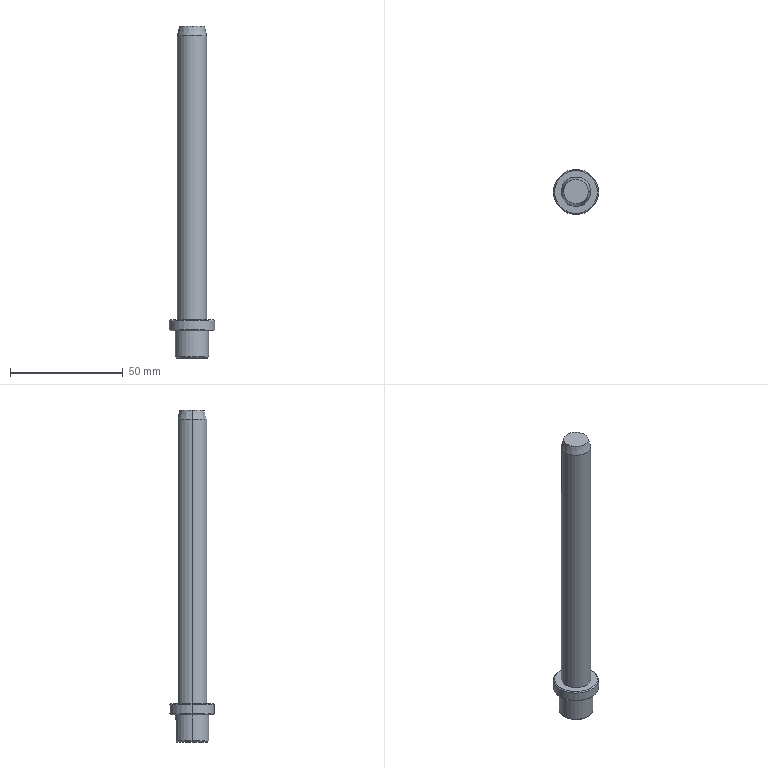Part | STEP file | 11-FG-B05711 | 1 solid | 23 faces | box 20 x 20 x 147 mm | volume 20612 mm3 | cone 9 | cylinder 7 | plane 7 | commonest cylinder face diameters 13 x3 15 x2 20 x2
STEP:
#1=CARTESIAN_POINT('',(9.5,0.,0.));
#2=VERTEX_POINT('',#1);
#3=CARTESIAN_POINT('',(-9.5,0.,0.));
#4=VERTEX_POINT('',#3);
#5=CARTESIAN_POINT('',(0.,0.,0.));
#6=DIRECTION('',(0.,0.,1.));
#7=DIRECTION('',(-1.,0.,0.));
#8=AXIS2_PLACEMENT_3D('',#5,#6,#7);
#9=CIRCLE('',#8,9.5);
#10=EDGE_CURVE('',#2,#4,#9,.T.);
#11=ORIENTED_EDGE('',*,*,#10,.F.);
#12=CARTESIAN_POINT('',(10.,0.,-0.5));
#13=VERTEX_POINT('',#12);
#14=CARTESIAN_POINT('',(10.,0.,-0.5));
#15=DIRECTION('',(0.7071,0.,-0.7071));
#16=VECTOR('',#15,1000.);
#17=LINE('',#14,#16);
#18=EDGE_CURVE('',#2,#13,#17,.T.);
#19=ORIENTED_EDGE('',*,*,#18,.T.);
#20=CARTESIAN_POINT('',(-10.,0.,-0.5));
#21=VERTEX_POINT('',#20);
#22=CARTESIAN_POINT('',(0.,0.,-0.5));
#23=DIRECTION('',(0.,0.,-1.));
#24=DIRECTION('',(-1.,0.,0.));
#25=AXIS2_PLACEMENT_3D('',#22,#23,#24);
#26=CIRCLE('',#25,10.);
#27=EDGE_CURVE('',#21,#13,#26,.T.);
#28=ORIENTED_EDGE('',*,*,#27,.F.);
#29=CARTESIAN_POINT('',(-10.,0.,-0.5));
#30=DIRECTION('',(-0.7071,0.,-0.7071));
#31=VECTOR('',#30,1000.);
#32=LINE('',#29,#31);
#33=EDGE_CURVE('',#4,#21,#32,.T.);
#34=ORIENTED_EDGE('',*,*,#33,.F.);
#35=EDGE_LOOP('',(#11,#19,#28,#34));
#36=FACE_OUTER_BOUND('',#35,.T.);
#37=CARTESIAN_POINT('',(0.,0.,-0.5));
#38=DIRECTION('',(0.,0.,-1.));
#39=DIRECTION('',(-1.,0.,0.));
#40=AXIS2_PLACEMENT_3D('',#37,#38,#39);
#41=CONICAL_SURFACE('',#40,10.,0.7854);
#42=ADVANCED_FACE('',(#36),#41,.T.);
#43=CARTESIAN_POINT('',(-9.5,0.,-5.));
#44=VERTEX_POINT('',#43);
#45=CARTESIAN_POINT('',(9.5,0.,-5.));
#46=VERTEX_POINT('',#45);
#47=CARTESIAN_POINT('',(0.,0.,-5.));
#48=DIRECTION('',(0.,0.,-1.));
#49=DIRECTION('',(-1.,0.,0.));
#50=AXIS2_PLACEMENT_3D('',#47,#48,#49);
#51=CIRCLE('',#50,9.5);
#52=EDGE_CURVE('',#44,#46,#51,.T.);
#53=ORIENTED_EDGE('',*,*,#52,.F.);
#54=CARTESIAN_POINT('',(-10.,0.,-4.5));
#55=VERTEX_POINT('',#54);
#56=CARTESIAN_POINT('',(-9.5,0.,-5.));
#57=DIRECTION('',(-0.7071,0.,0.7071));
#58=VECTOR('',#57,1000.);
#59=LINE('',#56,#58);
#60=EDGE_CURVE('',#44,#55,#59,.T.);
#61=ORIENTED_EDGE('',*,*,#60,.T.);
#62=CARTESIAN_POINT('',(10.,0.,-4.5));
#63=VERTEX_POINT('',#62);
#64=CARTESIAN_POINT('',(0.,0.,-4.5));
#65=DIRECTION('',(0.,0.,1.));
#66=DIRECTION('',(-1.,0.,0.));
#67=AXIS2_PLACEMENT_3D('',#64,#65,#66);
#68=CIRCLE('',#67,10.);
#69=EDGE_CURVE('',#63,#55,#68,.T.);
#70=ORIENTED_EDGE('',*,*,#69,.F.);
#71=CARTESIAN_POINT('',(9.5,0.,-5.));
#72=DIRECTION('',(0.7071,0.,0.7071));
#73=VECTOR('',#72,1000.);
#74=LINE('',#71,#73);
#75=EDGE_CURVE('',#46,#63,#74,.T.);
#76=ORIENTED_EDGE('',*,*,#75,.F.);
#77=EDGE_LOOP('',(#53,#61,#70,#76));
#78=FACE_OUTER_BOUND('',#77,.T.);
#79=CARTESIAN_POINT('',(0.,0.,-5.));
#80=DIRECTION('',(0.,0.,1.));
#81=DIRECTION('',(1.,0.,0.));
#82=AXIS2_PLACEMENT_3D('',#79,#80,#81);
#83=CONICAL_SURFACE('',#82,9.5,0.7854);
#84=ADVANCED_FACE('',(#78),#83,.T.);
#85=CARTESIAN_POINT('',(-7.,0.,-17.));
#86=VERTEX_POINT('',#85);
#87=CARTESIAN_POINT('',(0.,7.,-17.));
#88=VERTEX_POINT('',#87);
#89=CARTESIAN_POINT('',(0.,0.,-17.));
#90=DIRECTION('',(0.,0.,-1.));
#91=DIRECTION('',(-1.,0.,0.));
#92=AXIS2_PLACEMENT_3D('',#89,#90,#91);
#93=CIRCLE('',#92,7.);
#94=EDGE_CURVE('',#86,#88,#93,.T.);
#95=ORIENTED_EDGE('',*,*,#94,.F.);
#96=CARTESIAN_POINT('',(-7.5,0.,-16.5));
#97=VERTEX_POINT('',#96);
#98=CARTESIAN_POINT('',(-7.,0.,-17.));
#99=DIRECTION('',(-0.7071,0.,0.7071));
#100=VECTOR('',#99,1000.);
#101=LINE('',#98,#100);
#102=EDGE_CURVE('',#86,#97,#101,.T.);
#103=ORIENTED_EDGE('',*,*,#102,.T.);
#104=CARTESIAN_POINT('',(-2.693,7.,-16.5));
#105=VERTEX_POINT('',#104);
#106=CARTESIAN_POINT('',(0.,0.,-16.5));
#107=DIRECTION('',(0.,0.,1.));
#108=DIRECTION('',(-1.,0.,0.));
#109=AXIS2_PLACEMENT_3D('',#106,#107,#108);
#110=CIRCLE('',#109,7.5);
#111=EDGE_CURVE('',#105,#97,#110,.T.);
#112=ORIENTED_EDGE('',*,*,#111,.F.);
#113=CARTESIAN_POINT('',(0.,7.,-17.));
#114=CARTESIAN_POINT('',(-0.4603,7.,-17.));
#115=CARTESIAN_POINT('',(-0.9154,7.,-16.954));
#116=CARTESIAN_POINT('',(-1.816,7.,-16.782));
#117=CARTESIAN_POINT('',(-2.263,7.,-16.654));
#118=CARTESIAN_POINT('',(-2.693,7.,-16.5));
#119=B_SPLINE_CURVE_WITH_KNOTS('',3,(#113,#114,#115,#116,#117,#118),.UNSPECIFIED.,.F.,.F.,(4,2,4),(0.008783,0.01014,0.0115),.UNSPECIFIED.);
#120=EDGE_CURVE('',#88,#105,#119,.T.);
#121=ORIENTED_EDGE('',*,*,#120,.F.);
#122=EDGE_LOOP('',(#95,#103,#112,#121));
#123=FACE_OUTER_BOUND('',#122,.T.);
#124=CARTESIAN_POINT('',(0.,0.,-17.));
#125=DIRECTION('',(0.,0.,1.));
#126=DIRECTION('',(1.,0.,0.));
#127=AXIS2_PLACEMENT_3D('',#124,#125,#126);
#128=CONICAL_SURFACE('',#127,7.,0.7854);
#129=ADVANCED_FACE('',(#123),#128,.T.);
#130=ORIENTED_EDGE('',*,*,#102,.F.);
#131=CARTESIAN_POINT('',(7.,0.,-17.));
#132=VERTEX_POINT('',#131);
#133=CARTESIAN_POINT('',(0.,0.,-17.));
#134=DIRECTION('',(0.,0.,-1.));
#135=DIRECTION('',(-1.,0.,0.));
#136=AXIS2_PLACEMENT_3D('',#133,#134,#135);
#137=CIRCLE('',#136,7.);
#138=EDGE_CURVE('',#132,#86,#137,.T.);
#139=ORIENTED_EDGE('',*,*,#138,.F.);
#140=CARTESIAN_POINT('',(7.5,0.,-16.5));
#141=VERTEX_POINT('',#140);
#142=CARTESIAN_POINT('',(7.,0.,-17.));
#143=DIRECTION('',(0.7071,0.,0.7071));
#144=VECTOR('',#143,1000.);
#145=LINE('',#142,#144);
#146=EDGE_CURVE('',#132,#141,#145,.T.);
#147=ORIENTED_EDGE('',*,*,#146,.T.);
#148=CARTESIAN_POINT('',(0.,0.,-16.5));
#149=DIRECTION('',(0.,0.,1.));
#150=DIRECTION('',(-1.,0.,0.));
#151=AXIS2_PLACEMENT_3D('',#148,#149,#150);
#152=CIRCLE('',#151,7.5);
#153=EDGE_CURVE('',#97,#141,#152,.T.);
#154=ORIENTED_EDGE('',*,*,#153,.F.);
#155=EDGE_LOOP('',(#130,#139,#147,#154));
#156=FACE_OUTER_BOUND('',#155,.T.);
#157=CARTESIAN_POINT('',(0.,0.,-17.));
#158=DIRECTION('',(0.,0.,1.));
#159=DIRECTION('',(1.,0.,0.));
#160=AXIS2_PLACEMENT_3D('',#157,#158,#159);
#161=CONICAL_SURFACE('',#160,7.,0.7854);
#162=ADVANCED_FACE('',(#156),#161,.T.);
#163=ORIENTED_EDGE('',*,*,#111,.T.);
#164=CARTESIAN_POINT('',(-7.5,0.,-5.));
#165=VERTEX_POINT('',#164);
#166=CARTESIAN_POINT('',(-7.5,0.,-17.));
#167=DIRECTION('',(0.,0.,1.));
#168=VECTOR('',#167,1000.);
#169=LINE('',#166,#168);
#170=EDGE_CURVE('',#97,#165,#169,.T.);
#171=ORIENTED_EDGE('',*,*,#170,.T.);
#172=CARTESIAN_POINT('',(7.5,0.,-5.));
#173=VERTEX_POINT('',#172);
#174=CARTESIAN_POINT('',(0.,0.,-5.));
#175=DIRECTION('',(0.,0.,-1.));
#176=DIRECTION('',(-1.,0.,0.));
#177=AXIS2_PLACEMENT_3D('',#174,#175,#176);
#178=CIRCLE('',#177,7.5);
#179=EDGE_CURVE('',#165,#173,#178,.T.);
#180=ORIENTED_EDGE('',*,*,#179,.T.);
#181=CARTESIAN_POINT('',(7.5,0.,-17.));
#182=DIRECTION('',(0.,0.,1.));
#183=VECTOR('',#182,1000.);
#184=LINE('',#181,#183);
#185=EDGE_CURVE('',#141,#173,#184,.T.);
#186=ORIENTED_EDGE('',*,*,#185,.F.);
#187=CARTESIAN_POINT('',(2.693,7.,-16.5));
#188=VERTEX_POINT('',#187);
#189=CARTESIAN_POINT('',(0.,0.,-16.5));
#190=DIRECTION('',(0.,0.,1.));
#191=DIRECTION('',(-1.,0.,0.));
#192=AXIS2_PLACEMENT_3D('',#189,#190,#191);
#193=CIRCLE('',#192,7.5);
#194=EDGE_CURVE('',#141,#188,#193,.T.);
#195=ORIENTED_EDGE('',*,*,#194,.T.);
#196=CARTESIAN_POINT('',(2.693,7.,-7.));
#197=VERTEX_POINT('',#196);
#198=CARTESIAN_POINT('',(2.693,7.,-17.));
#199=DIRECTION('',(0.,0.,1.));
#200=VECTOR('',#199,1000.);
#201=LINE('',#198,#200);
#202=EDGE_CURVE('',#188,#197,#201,.T.);
#203=ORIENTED_EDGE('',*,*,#202,.T.);
#204=CARTESIAN_POINT('',(-2.693,7.,-7.));
#205=VERTEX_POINT('',#204);
#206=CARTESIAN_POINT('',(0.,0.,-7.));
#207=DIRECTION('',(0.,0.,-1.));
#208=DIRECTION('',(-1.,0.,0.));
#209=AXIS2_PLACEMENT_3D('',#206,#207,#208);
#210=CIRCLE('',#209,7.5);
#211=EDGE_CURVE('',#205,#197,#210,.T.);
#212=ORIENTED_EDGE('',*,*,#211,.F.);
#213=CARTESIAN_POINT('',(-2.693,7.,-17.));
#214=DIRECTION('',(0.,0.,-1.));
#215=VECTOR('',#214,1000.);
#216=LINE('',#213,#215);
#217=EDGE_CURVE('',#205,#105,#216,.T.);
#218=ORIENTED_EDGE('',*,*,#217,.T.);
#219=EDGE_LOOP('',(#163,#171,#180,#186,#195,#203,#212,#218));
#220=FACE_OUTER_BOUND('',#219,.T.);
#221=CARTESIAN_POINT('',(0.,0.,-17.));
#222=DIRECTION('',(0.,0.,1.));
#223=DIRECTION('',(1.,0.,0.));
#224=AXIS2_PLACEMENT_3D('',#221,#222,#223);
#225=CYLINDRICAL_SURFACE('',#224,7.5);
#226=ADVANCED_FACE('',(#220),#225,.T.);
#227=ORIENTED_EDGE('',*,*,#69,.T.);
#228=CARTESIAN_POINT('',(-10.,0.,-5.));
#229=DIRECTION('',(0.,0.,1.));
#230=VECTOR('',#229,1000.);
#231=LINE('',#228,#230);
#232=EDGE_CURVE('',#55,#21,#231,.T.);
#233=ORIENTED_EDGE('',*,*,#232,.T.);
#234=ORIENTED_EDGE('',*,*,#27,.T.);
#235=CARTESIAN_POINT('',(10.,0.,-5.));
#236=DIRECTION('',(0.,0.,1.));
#237=VECTOR('',#236,1000.);
#238=LINE('',#235,#237);
#239=EDGE_CURVE('',#63,#13,#238,.T.);
#240=ORIENTED_EDGE('',*,*,#239,.F.);
#241=EDGE_LOOP('',(#227,#233,#234,#240));
#242=FACE_OUTER_BOUND('',#241,.T.);
#243=CARTESIAN_POINT('',(0.,0.,-5.));
#244=DIRECTION('',(0.,0.,1.));
#245=DIRECTION('',(1.,0.,0.));
#246=AXIS2_PLACEMENT_3D('',#243,#244,#245);
#247=CYLINDRICAL_SURFACE('',#246,10.);
#248=ADVANCED_FACE('',(#242),#247,.T.);
#249=CARTESIAN_POINT('',(5.428,0.,130.));
#250=VERTEX_POINT('',#249);
#251=CARTESIAN_POINT('',(-5.428,0.,130.));
#252=VERTEX_POINT('',#251);
#253=CARTESIAN_POINT('',(0.,0.,130.));
#254=DIRECTION('',(0.,0.,1.));
#255=DIRECTION('',(1.,0.,0.));
#256=AXIS2_PLACEMENT_3D('',#253,#254,#255);
#257=CIRCLE('',#256,5.428);
#258=EDGE_CURVE('',#250,#252,#257,.T.);
#259=ORIENTED_EDGE('',*,*,#258,.F.);
#260=CARTESIAN_POINT('',(6.5,0.,126.));
#261=VERTEX_POINT('',#260);
#262=CARTESIAN_POINT('',(5.428,0.,130.));
#263=DIRECTION('',(0.2588,0.,-0.9659));
#264=VECTOR('',#263,1000.);
#265=LINE('',#262,#264);
#266=EDGE_CURVE('',#250,#261,#265,.T.);
#267=ORIENTED_EDGE('',*,*,#266,.T.);
#268=CARTESIAN_POINT('',(2.5,6.,126.));
#269=VERTEX_POINT('',#268);
#270=CARTESIAN_POINT('',(0.,0.,126.));
#271=DIRECTION('',(0.,0.,-1.));
#272=DIRECTION('',(1.,0.,0.));
#273=AXIS2_PLACEMENT_3D('',#270,#271,#272);
#274=CIRCLE('',#273,6.5);
#275=EDGE_CURVE('',#269,#261,#274,.T.);
#276=ORIENTED_EDGE('',*,*,#275,.F.);
#277=CARTESIAN_POINT('',(-2.5,6.,126.));
#278=VERTEX_POINT('',#277);
#279=CARTESIAN_POINT('',(2.5,6.,126.));
#280=CARTESIAN_POINT('',(2.346,6.,126.221));
#281=CARTESIAN_POINT('',(2.185,6.,126.435));
#282=CARTESIAN_POINT('',(1.84,6.,126.844));
#283=CARTESIAN_POINT('',(1.657,6.,127.039));
#284=CARTESIAN_POINT('',(1.253,6.,127.395));
#285=CARTESIAN_POINT('',(1.031,6.,127.556));
#286=CARTESIAN_POINT('',(0.6671,6.,127.733));
#287=CARTESIAN_POINT('',(0.5384,6.,127.781));
#288=CARTESIAN_POINT('',(0.2764,6.,127.848));
#289=CARTESIAN_POINT('',(0.1417,6.,127.866));
#290=CARTESIAN_POINT('',(-0.1312,6.,127.866));
#291=CARTESIAN_POINT('',(-0.265,6.,127.85));
#292=CARTESIAN_POINT('',(-0.5279,6.,127.785));
#293=CARTESIAN_POINT('',(-0.6568,6.,127.737));
#294=CARTESIAN_POINT('',(-1.022,6.,127.561));
#295=CARTESIAN_POINT('',(-1.245,6.,127.401));
#296=CARTESIAN_POINT('',(-1.65,6.,127.046));
#297=CARTESIAN_POINT('',(-1.835,6.,126.85));
#298=CARTESIAN_POINT('',(-2.184,6.,126.437));
#299=CARTESIAN_POINT('',(-2.346,6.,126.221));
#300=CARTESIAN_POINT('',(-2.5,6.,126.));
#301=B_SPLINE_CURVE_WITH_KNOTS('',3,(#279,#280,#281,#282,#283,#284,#285,#286,#287,#288,#289,#290,#291,#292,#293,#294,#295,#296,#297,#298,#299,#300),.UNSPECIFIED.,.F.,.F.,(4,2,2,2,2,2,2,2,2,2,4),(0.007754,0.008553,0.009351,0.01015,0.01055,0.01095,0.01135,0.01175,0.01254,0.01334,0.01414),.UNSPECIFIED.);
#302=EDGE_CURVE('',#269,#278,#301,.T.);
#303=ORIENTED_EDGE('',*,*,#302,.T.);
#304=CARTESIAN_POINT('',(-6.5,0.,126.));
#305=VERTEX_POINT('',#304);
#306=CARTESIAN_POINT('',(0.,0.,126.));
#307=DIRECTION('',(0.,0.,-1.));
#308=DIRECTION('',(1.,0.,0.));
#309=AXIS2_PLACEMENT_3D('',#306,#307,#308);
#310=CIRCLE('',#309,6.5);
#311=EDGE_CURVE('',#305,#278,#310,.T.);
#312=ORIENTED_EDGE('',*,*,#311,.F.);
#313=CARTESIAN_POINT('',(-5.428,0.,130.));
#314=DIRECTION('',(-0.2588,0.,-0.9659));
#315=VECTOR('',#314,1000.);
#316=LINE('',#313,#315);
#317=EDGE_CURVE('',#252,#305,#316,.T.);
#318=ORIENTED_EDGE('',*,*,#317,.F.);
#319=EDGE_LOOP('',(#259,#267,#276,#303,#312,#318));
#320=FACE_OUTER_BOUND('',#319,.T.);
#321=CARTESIAN_POINT('',(0.,0.,130.));
#322=DIRECTION('',(0.,0.,-1.));
#323=DIRECTION('',(-1.,0.,0.));
#324=AXIS2_PLACEMENT_3D('',#321,#322,#323);
#325=CONICAL_SURFACE('',#324,5.428,0.2618);
#326=ADVANCED_FACE('',(#320),#325,.T.);
#327=ORIENTED_EDGE('',*,*,#275,.T.);
#328=CARTESIAN_POINT('',(6.5,0.,0.));
#329=VERTEX_POINT('',#328);
#330=CARTESIAN_POINT('',(6.5,0.,130.));
#331=DIRECTION('',(0.,0.,-1.));
#332=VECTOR('',#331,1000.);
#333=LINE('',#330,#332);
#334=EDGE_CURVE('',#261,#329,#333,.T.);
#335=ORIENTED_EDGE('',*,*,#334,.T.);
#336=CARTESIAN_POINT('',(2.5,6.,0.));
#337=VERTEX_POINT('',#336);
#338=CARTESIAN_POINT('',(0.,0.,0.));
#339=DIRECTION('',(0.,0.,-1.));
#340=DIRECTION('',(-1.,0.,0.));
#341=AXIS2_PLACEMENT_3D('',#338,#339,#340);
#342=CIRCLE('',#341,6.5);
#343=EDGE_CURVE('',#337,#329,#342,.T.);
#344=ORIENTED_EDGE('',*,*,#343,.F.);
#345=CARTESIAN_POINT('',(2.5,6.,130.));
#346=DIRECTION('',(0.,0.,-1.));
#347=VECTOR('',#346,1000.);
#348=LINE('',#345,#347);
#349=EDGE_CURVE('',#269,#337,#348,.T.);
#350=ORIENTED_EDGE('',*,*,#349,.F.);
#351=EDGE_LOOP('',(#327,#335,#344,#350));
#352=FACE_OUTER_BOUND('',#351,.T.);
#353=CARTESIAN_POINT('',(0.,0.,130.));
#354=DIRECTION('',(0.,0.,-1.));
#355=DIRECTION('',(-1.,0.,0.));
#356=AXIS2_PLACEMENT_3D('',#353,#354,#355);
#357=CYLINDRICAL_SURFACE('',#356,6.5);
#358=ADVANCED_FACE('',(#352),#357,.T.);
#359=ORIENTED_EDGE('',*,*,#334,.F.);
#360=CARTESIAN_POINT('',(0.,0.,126.));
#361=DIRECTION('',(0.,0.,-1.));
#362=DIRECTION('',(1.,0.,0.));
#363=AXIS2_PLACEMENT_3D('',#360,#361,#362);
#364=CIRCLE('',#363,6.5);
#365=EDGE_CURVE('',#261,#305,#364,.T.);
#366=ORIENTED_EDGE('',*,*,#365,.T.);
#367=CARTESIAN_POINT('',(-6.5,0.,0.));
#368=VERTEX_POINT('',#367);
#369=CARTESIAN_POINT('',(-6.5,0.,130.));
#370=DIRECTION('',(0.,0.,-1.));
#371=VECTOR('',#370,1000.);
#372=LINE('',#369,#371);
#373=EDGE_CURVE('',#305,#368,#372,.T.);
#374=ORIENTED_EDGE('',*,*,#373,.T.);
#375=CARTESIAN_POINT('',(0.,0.,0.));
#376=DIRECTION('',(0.,0.,-1.));
#377=DIRECTION('',(-1.,0.,0.));
#378=AXIS2_PLACEMENT_3D('',#375,#376,#377);
#379=CIRCLE('',#378,6.5);
#380=EDGE_CURVE('',#329,#368,#379,.T.);
#381=ORIENTED_EDGE('',*,*,#380,.F.);
#382=EDGE_LOOP('',(#359,#366,#374,#381));
#383=FACE_OUTER_BOUND('',#382,.T.);
#384=CARTESIAN_POINT('',(0.,0.,130.));
#385=DIRECTION('',(0.,0.,-1.));
#386=DIRECTION('',(-1.,0.,0.));
#387=AXIS2_PLACEMENT_3D('',#384,#385,#386);
#388=CYLINDRICAL_SURFACE('',#387,6.5);
#389=ADVANCED_FACE('',(#383),#388,.T.);
#390=ORIENTED_EDGE('',*,*,#373,.F.);
#391=ORIENTED_EDGE('',*,*,#311,.T.);
#392=CARTESIAN_POINT('',(-2.5,6.,0.));
#393=VERTEX_POINT('',#392);
#394=CARTESIAN_POINT('',(-2.5,6.,130.));
#395=DIRECTION('',(0.,0.,1.));
#396=VECTOR('',#395,1000.);
#397=LINE('',#394,#396);
#398=EDGE_CURVE('',#393,#278,#397,.T.);
#399=ORIENTED_EDGE('',*,*,#398,.F.);
#400=CARTESIAN_POINT('',(0.,0.,0.));
#401=DIRECTION('',(0.,0.,-1.));
#402=DIRECTION('',(-1.,0.,0.));
#403=AXIS2_PLACEMENT_3D('',#400,#401,#402);
#404=CIRCLE('',#403,6.5);
#405=EDGE_CURVE('',#368,#393,#404,.T.);
#406=ORIENTED_EDGE('',*,*,#405,.F.);
#407=EDGE_LOOP('',(#390,#391,#399,#406));
#408=FACE_OUTER_BOUND('',#407,.T.);
#409=CARTESIAN_POINT('',(0.,0.,130.));
#410=DIRECTION('',(0.,0.,-1.));
#411=DIRECTION('',(-1.,0.,0.));
#412=AXIS2_PLACEMENT_3D('',#409,#410,#411);
#413=CYLINDRICAL_SURFACE('',#412,6.5);
#414=ADVANCED_FACE('',(#408),#413,.T.);
#415=ORIENTED_EDGE('',*,*,#266,.F.);
#416=CARTESIAN_POINT('',(0.,0.,130.));
#417=DIRECTION('',(0.,0.,1.));
#418=DIRECTION('',(1.,0.,0.));
#419=AXIS2_PLACEMENT_3D('',#416,#417,#418);
#420=CIRCLE('',#419,5.428);
#421=EDGE_CURVE('',#252,#250,#420,.T.);
#422=ORIENTED_EDGE('',*,*,#421,.F.);
#423=ORIENTED_EDGE('',*,*,#317,.T.);
#424=ORIENTED_EDGE('',*,*,#365,.F.);
#425=EDGE_LOOP('',(#415,#422,#423,#424));
#426=FACE_OUTER_BOUND('',#425,.T.);
#427=CARTESIAN_POINT('',(0.,0.,130.));
#428=DIRECTION('',(0.,0.,-1.));
#429=DIRECTION('',(-1.,0.,0.));
#430=AXIS2_PLACEMENT_3D('',#427,#428,#429);
#431=CONICAL_SURFACE('',#430,5.428,0.2618);
#432=ADVANCED_FACE('',(#426),#431,.T.);
#433=CARTESIAN_POINT('',(0.,0.,-5.));
#434=DIRECTION('',(0.,0.,-1.));
#435=DIRECTION('',(-1.,0.,0.));
#436=AXIS2_PLACEMENT_3D('',#433,#434,#435);
#437=CIRCLE('',#436,9.5);
#438=EDGE_CURVE('',#46,#44,#437,.T.);
#439=ORIENTED_EDGE('',*,*,#438,.T.);
#440=ORIENTED_EDGE('',*,*,#52,.T.);
#441=EDGE_LOOP('',(#439,#440));
#442=FACE_OUTER_BOUND('',#441,.T.);
#443=CARTESIAN_POINT('',(0.,0.,-5.));
#444=DIRECTION('',(0.,0.,-1.));
#445=DIRECTION('',(-1.,0.,0.));
#446=AXIS2_PLACEMENT_3D('',#443,#444,#445);
#447=CIRCLE('',#446,7.5);
#448=EDGE_CURVE('',#173,#165,#447,.T.);
#449=ORIENTED_EDGE('',*,*,#448,.F.);
#450=ORIENTED_EDGE('',*,*,#179,.F.);
#451=EDGE_LOOP('',(#449,#450));
#452=FACE_BOUND('',#451,.T.);
#453=CARTESIAN_POINT('',(0.,0.,-5.));
#454=DIRECTION('',(0.,0.,-1.));
#455=DIRECTION('',(-1.,0.,0.));
#456=AXIS2_PLACEMENT_3D('',#453,#454,#455);
#457=PLANE('',#456);
#458=ADVANCED_FACE('',(#442,#452),#457,.T.);
#459=ORIENTED_EDGE('',*,*,#421,.T.);
#460=ORIENTED_EDGE('',*,*,#258,.T.);
#461=EDGE_LOOP('',(#459,#460));
#462=FACE_OUTER_BOUND('',#461,.T.);
#463=CARTESIAN_POINT('',(0.,0.,130.));
#464=DIRECTION('',(0.,0.,1.));
#465=DIRECTION('',(1.,0.,0.));
#466=AXIS2_PLACEMENT_3D('',#463,#464,#465);
#467=PLANE('',#466);
#468=ADVANCED_FACE('',(#462),#467,.T.);
#469=CARTESIAN_POINT('',(0.,0.,0.));
#470=DIRECTION('',(0.,0.,1.));
#471=DIRECTION('',(-1.,0.,0.));
#472=AXIS2_PLACEMENT_3D('',#469,#470,#471);
#473=CIRCLE('',#472,9.5);
#474=EDGE_CURVE('',#4,#2,#473,.T.);
#475=ORIENTED_EDGE('',*,*,#474,.T.);
#476=ORIENTED_EDGE('',*,*,#10,.T.);
#477=EDGE_LOOP('',(#475,#476));
#478=FACE_OUTER_BOUND('',#477,.T.);
#479=ORIENTED_EDGE('',*,*,#343,.T.);
#480=ORIENTED_EDGE('',*,*,#380,.T.);
#481=ORIENTED_EDGE('',*,*,#405,.T.);
#482=CARTESIAN_POINT('',(-7.766,6.,0.));
#483=DIRECTION('',(1.,0.,0.));
#484=VECTOR('',#483,1000.);
#485=LINE('',#482,#484);
#486=EDGE_CURVE('',#393,#337,#485,.T.);
#487=ORIENTED_EDGE('',*,*,#486,.T.);
#488=EDGE_LOOP('',(#479,#480,#481,#487));
#489=FACE_BOUND('',#488,.T.);
#490=CARTESIAN_POINT('',(0.,0.,0.));
#491=DIRECTION('',(0.,0.,-1.));
#492=DIRECTION('',(-1.,0.,0.));
#493=AXIS2_PLACEMENT_3D('',#490,#491,#492);
#494=PLANE('',#493);
#495=ADVANCED_FACE('',(#478,#489),#494,.F.);
#496=ORIENTED_EDGE('',*,*,#232,.F.);
#497=CARTESIAN_POINT('',(0.,0.,-4.5));
#498=DIRECTION('',(0.,0.,1.));
#499=DIRECTION('',(-1.,0.,0.));
#500=AXIS2_PLACEMENT_3D('',#497,#498,#499);
#501=CIRCLE('',#500,10.);
#502=EDGE_CURVE('',#55,#63,#501,.T.);
#503=ORIENTED_EDGE('',*,*,#502,.T.);
#504=ORIENTED_EDGE('',*,*,#239,.T.);
#505=CARTESIAN_POINT('',(0.,0.,-0.5));
#506=DIRECTION('',(0.,0.,-1.));
#507=DIRECTION('',(-1.,0.,0.));
#508=AXIS2_PLACEMENT_3D('',#505,#506,#507);
#509=CIRCLE('',#508,10.);
#510=EDGE_CURVE('',#13,#21,#509,.T.);
#511=ORIENTED_EDGE('',*,*,#510,.T.);
#512=EDGE_LOOP('',(#496,#503,#504,#511));
#513=FACE_OUTER_BOUND('',#512,.T.);
#514=CARTESIAN_POINT('',(0.,0.,-5.));
#515=DIRECTION('',(0.,0.,1.));
#516=DIRECTION('',(1.,0.,0.));
#517=AXIS2_PLACEMENT_3D('',#514,#515,#516);
#518=CYLINDRICAL_SURFACE('',#517,10.);
#519=ADVANCED_FACE('',(#513),#518,.T.);
#520=ORIENTED_EDGE('',*,*,#170,.F.);
#521=ORIENTED_EDGE('',*,*,#153,.T.);
#522=ORIENTED_EDGE('',*,*,#185,.T.);
#523=ORIENTED_EDGE('',*,*,#448,.T.);
#524=EDGE_LOOP('',(#520,#521,#522,#523));
#525=FACE_OUTER_BOUND('',#524,.T.);
#526=CARTESIAN_POINT('',(0.,0.,-17.));
#527=DIRECTION('',(0.,0.,1.));
#528=DIRECTION('',(1.,0.,0.));
#529=AXIS2_PLACEMENT_3D('',#526,#527,#528);
#530=CYLINDRICAL_SURFACE('',#529,7.5);
#531=ADVANCED_FACE('',(#525),#530,.T.);
#532=CARTESIAN_POINT('',(0.,0.,-17.));
#533=DIRECTION('',(0.,0.,-1.));
#534=DIRECTION('',(-1.,0.,0.));
#535=AXIS2_PLACEMENT_3D('',#532,#533,#534);
#536=CIRCLE('',#535,7.);
#537=EDGE_CURVE('',#88,#132,#536,.T.);
#538=ORIENTED_EDGE('',*,*,#537,.T.);
#539=ORIENTED_EDGE('',*,*,#138,.T.);
#540=ORIENTED_EDGE('',*,*,#94,.T.);
#541=EDGE_LOOP('',(#538,#539,#540));
#542=FACE_OUTER_BOUND('',#541,.T.);
#543=CARTESIAN_POINT('',(0.,0.,-17.));
#544=DIRECTION('',(0.,0.,-1.));
#545=DIRECTION('',(-1.,0.,0.));
#546=AXIS2_PLACEMENT_3D('',#543,#544,#545);
#547=PLANE('',#546);
#548=ADVANCED_FACE('',(#542),#547,.T.);
#549=ORIENTED_EDGE('',*,*,#349,.T.);
#550=ORIENTED_EDGE('',*,*,#486,.F.);
#551=ORIENTED_EDGE('',*,*,#398,.T.);
#552=ORIENTED_EDGE('',*,*,#302,.F.);
#553=EDGE_LOOP('',(#549,#550,#551,#552));
#554=FACE_OUTER_BOUND('',#553,.T.);
#555=CARTESIAN_POINT('',(-7.766,6.,130.));
#556=DIRECTION('',(0.,1.,0.));
#557=DIRECTION('',(0.,0.,1.));
#558=AXIS2_PLACEMENT_3D('',#555,#556,#557);
#559=PLANE('',#558);
#560=ADVANCED_FACE('',(#554),#559,.T.);
#561=ORIENTED_EDGE('',*,*,#146,.F.);
#562=ORIENTED_EDGE('',*,*,#537,.F.);
#563=CARTESIAN_POINT('',(2.693,7.,-16.5));
#564=CARTESIAN_POINT('',(2.258,7.,-16.656));
#565=CARTESIAN_POINT('',(1.818,7.,-16.781));
#566=CARTESIAN_POINT('',(1.145,7.,-16.91));
#567=CARTESIAN_POINT('',(0.919,7.,-16.944));
#568=CARTESIAN_POINT('',(0.4621,7.,-16.988));
#569=CARTESIAN_POINT('',(0.2303,7.,-17.));
#570=CARTESIAN_POINT('',(0.,7.,-17.));
#571=B_SPLINE_CURVE_WITH_KNOTS('',3,(#563,#564,#565,#566,#567,#568,#569,#570),.UNSPECIFIED.,.F.,.F.,(4,2,2,4),(0.006062,0.007422,0.008103,0.008783),.UNSPECIFIED.);
#572=EDGE_CURVE('',#188,#88,#571,.T.);
#573=ORIENTED_EDGE('',*,*,#572,.F.);
#574=ORIENTED_EDGE('',*,*,#194,.F.);
#575=EDGE_LOOP('',(#561,#562,#573,#574));
#576=FACE_OUTER_BOUND('',#575,.T.);
#577=CARTESIAN_POINT('',(0.,0.,-17.));
#578=DIRECTION('',(0.,0.,1.));
#579=DIRECTION('',(1.,0.,0.));
#580=AXIS2_PLACEMENT_3D('',#577,#578,#579);
#581=CONICAL_SURFACE('',#580,7.,0.7854);
#582=ADVANCED_FACE('',(#576),#581,.T.);
#583=ORIENTED_EDGE('',*,*,#60,.F.);
#584=ORIENTED_EDGE('',*,*,#438,.F.);
#585=ORIENTED_EDGE('',*,*,#75,.T.);
#586=ORIENTED_EDGE('',*,*,#502,.F.);
#587=EDGE_LOOP('',(#583,#584,#585,#586));
#588=FACE_OUTER_BOUND('',#587,.T.);
#589=CARTESIAN_POINT('',(0.,0.,-5.));
#590=DIRECTION('',(0.,0.,1.));
#591=DIRECTION('',(1.,0.,0.));
#592=AXIS2_PLACEMENT_3D('',#589,#590,#591);
#593=CONICAL_SURFACE('',#592,9.5,0.7854);
#594=ADVANCED_FACE('',(#588),#593,.T.);
#595=ORIENTED_EDGE('',*,*,#18,.F.);
#596=ORIENTED_EDGE('',*,*,#474,.F.);
#597=ORIENTED_EDGE('',*,*,#33,.T.);
#598=ORIENTED_EDGE('',*,*,#510,.F.);
#599=EDGE_LOOP('',(#595,#596,#597,#598));
#600=FACE_OUTER_BOUND('',#599,.T.);
#601=CARTESIAN_POINT('',(0.,0.,-0.5));
#602=DIRECTION('',(0.,0.,-1.));
#603=DIRECTION('',(-1.,0.,0.));
#604=AXIS2_PLACEMENT_3D('',#601,#602,#603);
#605=CONICAL_SURFACE('',#604,10.,0.7854);
#606=ADVANCED_FACE('',(#600),#605,.T.);
#607=ORIENTED_EDGE('',*,*,#211,.T.);
#608=CARTESIAN_POINT('',(10.363,7.,-7.));
#609=DIRECTION('',(-1.,0.,0.));
#610=VECTOR('',#609,1000.);
#611=LINE('',#608,#610);
#612=EDGE_CURVE('',#197,#205,#611,.T.);
#613=ORIENTED_EDGE('',*,*,#612,.T.);
#614=EDGE_LOOP('',(#607,#613));
#615=FACE_OUTER_BOUND('',#614,.T.);
#616=CARTESIAN_POINT('',(10.363,7.,-7.));
#617=DIRECTION('',(0.,0.,-1.));
#618=DIRECTION('',(-1.,0.,0.));
#619=AXIS2_PLACEMENT_3D('',#616,#617,#618);
#620=PLANE('',#619);
#621=ADVANCED_FACE('',(#615),#620,.T.);
#622=ORIENTED_EDGE('',*,*,#572,.T.);
#623=ORIENTED_EDGE('',*,*,#120,.T.);
#624=ORIENTED_EDGE('',*,*,#217,.F.);
#625=ORIENTED_EDGE('',*,*,#612,.F.);
#626=ORIENTED_EDGE('',*,*,#202,.F.);
#627=EDGE_LOOP('',(#622,#623,#624,#625,#626));
#628=FACE_OUTER_BOUND('',#627,.T.);
#629=CARTESIAN_POINT('',(10.363,7.,-7.));
#630=DIRECTION('',(0.,-1.,0.));
#631=DIRECTION('',(0.,0.,-1.));
#632=AXIS2_PLACEMENT_3D('',#629,#630,#631);
#633=PLANE('',#632);
#634=ADVANCED_FACE('',(#628),#633,.F.);
#635=CLOSED_SHELL('',(#42,#84,#129,#162,#226,#248,#326,#358,#389,#414,#432,#458,#468,#495,#519,#531,#548,#560,#582,#594,#606,#621,#634));
#636=MANIFOLD_SOLID_BREP('',#635);
#637=CARTESIAN_POINT('',(0.,0.,0.));
#638=DIRECTION('',(0.,0.,1.));
#639=DIRECTION('',(1.,0.,0.));
#640=AXIS2_PLACEMENT_3D('',#637,#638,#639);
#641=(LENGTH_UNIT()NAMED_UNIT(*)SI_UNIT(.MILLI.,.METRE.));
#642=UNCERTAINTY_MEASURE_WITH_UNIT(LENGTH_MEASURE(0.00001),#641,'','');
#643=(NAMED_UNIT(*)PLANE_ANGLE_UNIT()SI_UNIT($,.RADIAN.));
#644=(NAMED_UNIT(*)SI_UNIT($,.STERADIAN.)SOLID_ANGLE_UNIT());
#645=(GEOMETRIC_REPRESENTATION_CONTEXT(3)GLOBAL_UNCERTAINTY_ASSIGNED_CONTEXT((#642))GLOBAL_UNIT_ASSIGNED_CONTEXT((#641,#643,#644))REPRESENTATION_CONTEXT('',''));
#646=ADVANCED_BREP_SHAPE_REPRESENTATION('',(#636,#640),#645);